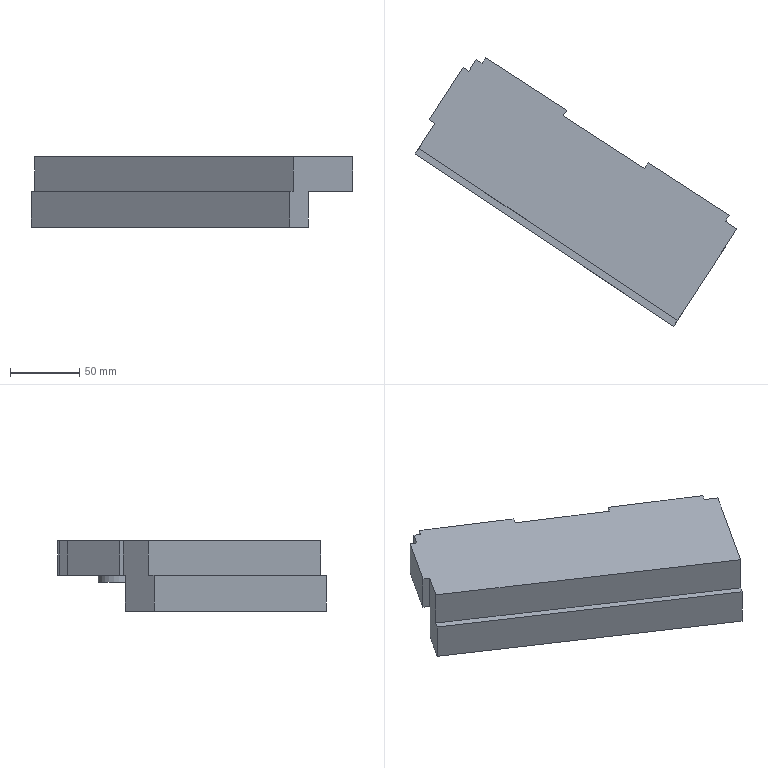Part | NX | features solid 2 | 1 solid | 30 faces | box 233.093 x 194.645 x 51 mm | volume 621496 mm3 | plane 24 | cylinder 4 | spline 2 | commonest cylinder face diameters 30 x4
STEP:
#1=CARTESIAN_POINT('',(545.617,534.28,20.));
#2=VERTEX_POINT('',#1);
#3=CARTESIAN_POINT('',(530.617,534.28,20.));
#4=DIRECTION('',(0.,0.,1.));
#5=DIRECTION('',(1.,0.,0.));
#6=AXIS2_PLACEMENT_3D('',#3,#4,#5);
#7=CIRCLE('',#6,15.);
#8=EDGE_CURVE('',#2,#2,#7,.F.);
#9=ORIENTED_EDGE('',*,*,#8,.F.);
#10=EDGE_LOOP('',(#9));
#11=FACE_BOUND('',#10,.T.);
#12=CARTESIAN_POINT('',(415.617,624.28,20.));
#13=VERTEX_POINT('',#12);
#14=CARTESIAN_POINT('',(400.617,624.28,20.));
#15=DIRECTION('',(0.,0.,1.));
#16=DIRECTION('',(1.,0.,0.));
#17=AXIS2_PLACEMENT_3D('',#14,#15,#16);
#18=CIRCLE('',#17,15.);
#19=EDGE_CURVE('',#13,#13,#18,.F.);
#20=ORIENTED_EDGE('',*,*,#19,.F.);
#21=EDGE_LOOP('',(#20));
#22=FACE_BOUND('',#21,.T.);
#23=CARTESIAN_POINT('',(391.424,667.003,20.));
#24=VERTEX_POINT('',#23);
#25=CARTESIAN_POINT('',(395.617,664.28,20.));
#26=VERTEX_POINT('',#25);
#27=CARTESIAN_POINT('',(-1256.754,1737.343,20.));
#28=DIRECTION('',(0.8387,-0.5446,0.));
#29=VECTOR('',#28,1000.);
#30=LINE('',#27,#29);
#31=EDGE_CURVE('',#24,#26,#30,.T.);
#32=ORIENTED_EDGE('',*,*,#31,.T.);
#33=CARTESIAN_POINT('',(398.341,668.473,20.));
#34=VERTEX_POINT('',#33);
#35=CARTESIAN_POINT('',(395.617,664.28,20.));
#36=DIRECTION('',(0.5446,0.8387,0.));
#37=VECTOR('',#36,1000.);
#38=LINE('',#35,#37);
#39=EDGE_CURVE('',#26,#34,#38,.T.);
#40=ORIENTED_EDGE('',*,*,#39,.T.);
#41=CARTESIAN_POINT('',(457.048,630.348,20.));
#42=VERTEX_POINT('',#41);
#43=CARTESIAN_POINT('',(406.727,663.027,20.));
#44=DIRECTION('',(0.8387,-0.5446,0.));
#45=VECTOR('',#44,1000.);
#46=LINE('',#43,#45);
#47=EDGE_CURVE('',#34,#42,#46,.T.);
#48=ORIENTED_EDGE('',*,*,#47,.T.);
#49=CARTESIAN_POINT('',(454.324,626.155,20.));
#50=VERTEX_POINT('',#49);
#51=CARTESIAN_POINT('',(454.324,626.155,20.));
#52=DIRECTION('',(0.5446,0.8387,0.));
#53=VECTOR('',#52,1000.);
#54=LINE('',#51,#53);
#55=EDGE_CURVE('',#50,#42,#54,.T.);
#56=ORIENTED_EDGE('',*,*,#55,.F.);
#57=CARTESIAN_POINT('',(513.031,588.03,20.));
#58=VERTEX_POINT('',#57);
#59=CARTESIAN_POINT('',(-1256.754,1737.343,20.));
#60=DIRECTION('',(0.8387,-0.5446,0.));
#61=VECTOR('',#60,1000.);
#62=LINE('',#59,#61);
#63=EDGE_CURVE('',#50,#58,#62,.T.);
#64=ORIENTED_EDGE('',*,*,#63,.T.);
#65=CARTESIAN_POINT('',(515.755,592.224,20.));
#66=VERTEX_POINT('',#65);
#67=CARTESIAN_POINT('',(513.031,588.03,20.));
#68=DIRECTION('',(0.5446,0.8387,0.));
#69=VECTOR('',#68,1000.);
#70=LINE('',#67,#69);
#71=EDGE_CURVE('',#58,#66,#70,.T.);
#72=ORIENTED_EDGE('',*,*,#71,.T.);
#73=CARTESIAN_POINT('',(574.461,554.099,20.));
#74=VERTEX_POINT('',#73);
#75=CARTESIAN_POINT('',(545.108,573.161,20.));
#76=DIRECTION('',(0.8387,-0.5446,0.));
#77=VECTOR('',#76,1000.);
#78=LINE('',#75,#77);
#79=EDGE_CURVE('',#66,#74,#78,.T.);
#80=ORIENTED_EDGE('',*,*,#79,.T.);
#81=CARTESIAN_POINT('',(571.738,549.906,20.));
#82=VERTEX_POINT('',#81);
#83=CARTESIAN_POINT('',(571.738,549.906,20.));
#84=DIRECTION('',(0.5446,0.8387,0.));
#85=VECTOR('',#84,1000.);
#86=LINE('',#83,#85);
#87=EDGE_CURVE('',#82,#74,#86,.T.);
#88=ORIENTED_EDGE('',*,*,#87,.F.);
#89=CARTESIAN_POINT('',(580.125,544.459,20.));
#90=VERTEX_POINT('',#89);
#91=CARTESIAN_POINT('',(-1256.754,1737.343,20.));
#92=DIRECTION('',(0.8387,-0.5446,0.));
#93=VECTOR('',#92,1000.);
#94=LINE('',#91,#93);
#95=EDGE_CURVE('',#82,#90,#94,.T.);
#96=ORIENTED_EDGE('',*,*,#95,.T.);
#97=CARTESIAN_POINT('',(547.874,494.797,20.));
#98=VERTEX_POINT('',#97);
#99=CARTESIAN_POINT('',(1248.625,1573.86,20.));
#100=DIRECTION('',(-0.5446,-0.8387,0.));
#101=VECTOR('',#100,1000.);
#102=LINE('',#99,#101);
#103=EDGE_CURVE('',#90,#98,#102,.T.);
#104=ORIENTED_EDGE('',*,*,#103,.T.);
#105=CARTESIAN_POINT('',(360.649,619.614,20.));
#106=VERTEX_POINT('',#105);
#107=CARTESIAN_POINT('',(547.874,494.797,20.));
#108=CARTESIAN_POINT('',(485.466,536.403,20.));
#109=CARTESIAN_POINT('',(423.057,578.008,20.));
#110=CARTESIAN_POINT('',(360.649,619.614,20.));
#111=B_SPLINE_CURVE_WITH_KNOTS('',3,(#107,#108,#109,#110),.UNSPECIFIED.,.F.,.F.,(4,4),(1.354,1.579),.UNSPECIFIED.);
#112=EDGE_CURVE('',#106,#98,#111,.F.);
#113=ORIENTED_EDGE('',*,*,#112,.F.);
#114=CARTESIAN_POINT('',(361.469,620.876,20.));
#115=VERTEX_POINT('',#114);
#116=CARTESIAN_POINT('',(1059.925,1696.404,20.));
#117=DIRECTION('',(-0.5446,-0.8387,0.));
#118=VECTOR('',#117,1000.);
#119=LINE('',#116,#118);
#120=EDGE_CURVE('',#115,#106,#119,.T.);
#121=ORIENTED_EDGE('',*,*,#120,.F.);
#122=CARTESIAN_POINT('',(357.276,623.599,20.));
#123=VERTEX_POINT('',#122);
#124=CARTESIAN_POINT('',(361.469,620.876,20.));
#125=DIRECTION('',(-0.8387,0.5446,0.));
#126=VECTOR('',#125,1000.);
#127=LINE('',#124,#126);
#128=EDGE_CURVE('',#115,#123,#127,.T.);
#129=ORIENTED_EDGE('',*,*,#128,.T.);
#130=CARTESIAN_POINT('',(381.784,661.34,20.));
#131=VERTEX_POINT('',#130);
#132=CARTESIAN_POINT('',(384.508,665.533,20.));
#133=DIRECTION('',(0.5446,0.8387,0.));
#134=VECTOR('',#133,1000.);
#135=LINE('',#132,#134);
#136=EDGE_CURVE('',#123,#131,#135,.T.);
#137=ORIENTED_EDGE('',*,*,#136,.T.);
#138=CARTESIAN_POINT('',(385.978,658.616,20.));
#139=VERTEX_POINT('',#138);
#140=CARTESIAN_POINT('',(385.978,658.616,20.));
#141=DIRECTION('',(-0.8387,0.5446,0.));
#142=VECTOR('',#141,1000.);
#143=LINE('',#140,#142);
#144=EDGE_CURVE('',#139,#131,#143,.T.);
#145=ORIENTED_EDGE('',*,*,#144,.F.);
#146=CARTESIAN_POINT('',(1059.925,1696.404,20.));
#147=DIRECTION('',(-0.5446,-0.8387,0.));
#148=VECTOR('',#147,1000.);
#149=LINE('',#146,#148);
#150=EDGE_CURVE('',#24,#139,#149,.T.);
#151=ORIENTED_EDGE('',*,*,#150,.F.);
#152=EDGE_LOOP('',(#32,#40,#48,#56,#64,#72,#80,#88,#96,#104,#113,#121,#129,#137,#145,#151));
#153=FACE_BOUND('',#152,.T.);
#154=CARTESIAN_POINT('',(515.617,559.28,20.));
#155=VERTEX_POINT('',#154);
#156=CARTESIAN_POINT('',(500.617,559.28,20.));
#157=DIRECTION('',(0.,0.,1.));
#158=DIRECTION('',(1.,0.,0.));
#159=AXIS2_PLACEMENT_3D('',#156,#157,#158);
#160=CIRCLE('',#159,15.);
#161=EDGE_CURVE('',#155,#155,#160,.F.);
#162=ORIENTED_EDGE('',*,*,#161,.F.);
#163=EDGE_LOOP('',(#162));
#164=FACE_BOUND('',#163,.T.);
#165=CARTESIAN_POINT('',(450.617,614.28,20.));
#166=VERTEX_POINT('',#165);
#167=CARTESIAN_POINT('',(435.617,614.28,20.));
#168=DIRECTION('',(0.,0.,1.));
#169=DIRECTION('',(1.,0.,0.));
#170=AXIS2_PLACEMENT_3D('',#167,#168,#169);
#171=CIRCLE('',#170,15.);
#172=EDGE_CURVE('',#166,#166,#171,.F.);
#173=ORIENTED_EDGE('',*,*,#172,.F.);
#174=EDGE_LOOP('',(#173));
#175=FACE_BOUND('',#174,.T.);
#176=CARTESIAN_POINT('',(369.22,631.927,20.));
#177=DIRECTION('',(0.,0.,1.));
#178=DIRECTION('',(1.,0.,0.));
#179=AXIS2_PLACEMENT_3D('',#176,#177,#178);
#180=PLANE('',#179);
#181=ADVANCED_FACE('',(#11,#22,#153,#164,#175),#180,.F.);
#182=ORIENTED_EDGE('',*,*,#95,.F.);
#183=CARTESIAN_POINT('',(571.738,549.906,45.));
#184=VERTEX_POINT('',#183);
#185=CARTESIAN_POINT('',(571.738,549.906,20.));
#186=DIRECTION('',(0.,0.,1.));
#187=VECTOR('',#186,1000.);
#188=LINE('',#185,#187);
#189=EDGE_CURVE('',#82,#184,#188,.T.);
#190=ORIENTED_EDGE('',*,*,#189,.T.);
#191=CARTESIAN_POINT('',(580.125,544.459,45.));
#192=VERTEX_POINT('',#191);
#193=CARTESIAN_POINT('',(-1256.754,1737.343,45.));
#194=DIRECTION('',(0.8387,-0.5446,0.));
#195=VECTOR('',#194,1000.);
#196=LINE('',#193,#195);
#197=EDGE_CURVE('',#184,#192,#196,.T.);
#198=ORIENTED_EDGE('',*,*,#197,.T.);
#199=CARTESIAN_POINT('',(580.125,544.459,70.));
#200=DIRECTION('',(0.,0.,1.));
#201=VECTOR('',#200,1000.);
#202=LINE('',#199,#201);
#203=EDGE_CURVE('',#90,#192,#202,.T.);
#204=ORIENTED_EDGE('',*,*,#203,.F.);
#205=EDGE_LOOP('',(#182,#190,#198,#204));
#206=FACE_BOUND('',#205,.T.);
#207=CARTESIAN_POINT('',(-1256.754,1737.343,70.));
#208=DIRECTION('',(0.5446,0.8387,0.));
#209=DIRECTION('',(-0.8387,0.5446,0.));
#210=AXIS2_PLACEMENT_3D('',#207,#208,#209);
#211=PLANE('',#210);
#212=ADVANCED_FACE('',(#206),#211,.T.);
#213=CARTESIAN_POINT('',(513.031,588.03,45.));
#214=VERTEX_POINT('',#213);
#215=CARTESIAN_POINT('',(513.031,588.03,20.));
#216=DIRECTION('',(0.,0.,-1.));
#217=VECTOR('',#216,1000.);
#218=LINE('',#215,#217);
#219=EDGE_CURVE('',#58,#214,#218,.F.);
#220=ORIENTED_EDGE('',*,*,#219,.F.);
#221=ORIENTED_EDGE('',*,*,#63,.F.);
#222=CARTESIAN_POINT('',(454.324,626.155,45.));
#223=VERTEX_POINT('',#222);
#224=CARTESIAN_POINT('',(454.324,626.155,20.));
#225=DIRECTION('',(0.,0.,1.));
#226=VECTOR('',#225,1000.);
#227=LINE('',#224,#226);
#228=EDGE_CURVE('',#50,#223,#227,.T.);
#229=ORIENTED_EDGE('',*,*,#228,.T.);
#230=CARTESIAN_POINT('',(-1256.754,1737.343,45.));
#231=DIRECTION('',(0.8387,-0.5446,0.));
#232=VECTOR('',#231,1000.);
#233=LINE('',#230,#232);
#234=EDGE_CURVE('',#223,#214,#233,.T.);
#235=ORIENTED_EDGE('',*,*,#234,.T.);
#236=EDGE_LOOP('',(#220,#221,#229,#235));
#237=FACE_BOUND('',#236,.T.);
#238=CARTESIAN_POINT('',(-1256.754,1737.343,70.));
#239=DIRECTION('',(0.5446,0.8387,0.));
#240=DIRECTION('',(-0.8387,0.5446,0.));
#241=AXIS2_PLACEMENT_3D('',#238,#239,#240);
#242=PLANE('',#241);
#243=ADVANCED_FACE('',(#237),#242,.T.);
#244=CARTESIAN_POINT('',(385.978,658.616,45.));
#245=VERTEX_POINT('',#244);
#246=CARTESIAN_POINT('',(385.978,658.616,20.));
#247=DIRECTION('',(0.,0.,1.));
#248=VECTOR('',#247,1000.);
#249=LINE('',#246,#248);
#250=EDGE_CURVE('',#139,#245,#249,.T.);
#251=ORIENTED_EDGE('',*,*,#250,.T.);
#252=CARTESIAN_POINT('',(391.424,667.003,45.));
#253=VERTEX_POINT('',#252);
#254=CARTESIAN_POINT('',(1059.925,1696.404,45.));
#255=DIRECTION('',(-0.5446,-0.8387,0.));
#256=VECTOR('',#255,1000.);
#257=LINE('',#254,#256);
#258=EDGE_CURVE('',#253,#245,#257,.T.);
#259=ORIENTED_EDGE('',*,*,#258,.F.);
#260=CARTESIAN_POINT('',(391.424,667.003,70.));
#261=DIRECTION('',(0.,0.,-1.));
#262=VECTOR('',#261,1000.);
#263=LINE('',#260,#262);
#264=EDGE_CURVE('',#253,#24,#263,.T.);
#265=ORIENTED_EDGE('',*,*,#264,.T.);
#266=ORIENTED_EDGE('',*,*,#150,.T.);
#267=EDGE_LOOP('',(#251,#259,#265,#266));
#268=FACE_BOUND('',#267,.T.);
#269=CARTESIAN_POINT('',(1059.925,1696.404,70.));
#270=DIRECTION('',(0.8387,-0.5446,0.));
#271=DIRECTION('',(0.5446,0.8387,0.));
#272=AXIS2_PLACEMENT_3D('',#269,#270,#271);
#273=PLANE('',#272);
#274=ADVANCED_FACE('',(#268),#273,.F.);
#275=CARTESIAN_POINT('',(395.617,664.28,45.));
#276=VERTEX_POINT('',#275);
#277=CARTESIAN_POINT('',(395.617,664.28,20.));
#278=DIRECTION('',(0.,0.,-1.));
#279=VECTOR('',#278,1000.);
#280=LINE('',#277,#279);
#281=EDGE_CURVE('',#26,#276,#280,.F.);
#282=ORIENTED_EDGE('',*,*,#281,.F.);
#283=ORIENTED_EDGE('',*,*,#31,.F.);
#284=ORIENTED_EDGE('',*,*,#264,.F.);
#285=CARTESIAN_POINT('',(-1256.754,1737.343,45.));
#286=DIRECTION('',(0.8387,-0.5446,0.));
#287=VECTOR('',#286,1000.);
#288=LINE('',#285,#287);
#289=EDGE_CURVE('',#253,#276,#288,.T.);
#290=ORIENTED_EDGE('',*,*,#289,.T.);
#291=EDGE_LOOP('',(#282,#283,#284,#290));
#292=FACE_BOUND('',#291,.T.);
#293=CARTESIAN_POINT('',(-1256.754,1737.343,70.));
#294=DIRECTION('',(0.5446,0.8387,0.));
#295=DIRECTION('',(-0.8387,0.5446,0.));
#296=AXIS2_PLACEMENT_3D('',#293,#294,#295);
#297=PLANE('',#296);
#298=ADVANCED_FACE('',(#292),#297,.T.);
#299=CARTESIAN_POINT('',(361.469,620.876,45.));
#300=VERTEX_POINT('',#299);
#301=CARTESIAN_POINT('',(349.755,602.839,45.));
#302=VERTEX_POINT('',#301);
#303=CARTESIAN_POINT('',(1059.925,1696.404,45.));
#304=DIRECTION('',(-0.5446,-0.8387,0.));
#305=VECTOR('',#304,1000.);
#306=LINE('',#303,#305);
#307=EDGE_CURVE('',#300,#302,#306,.T.);
#308=ORIENTED_EDGE('',*,*,#307,.F.);
#309=CARTESIAN_POINT('',(361.469,620.876,20.));
#310=DIRECTION('',(0.,0.,-1.));
#311=VECTOR('',#310,1000.);
#312=LINE('',#309,#311);
#313=EDGE_CURVE('',#115,#300,#312,.F.);
#314=ORIENTED_EDGE('',*,*,#313,.F.);
#315=ORIENTED_EDGE('',*,*,#120,.T.);
#316=CARTESIAN_POINT('',(360.649,619.614,-6.));
#317=VERTEX_POINT('',#316);
#318=CARTESIAN_POINT('',(360.649,619.614,-6.));
#319=DIRECTION('',(0.,0.,1.));
#320=VECTOR('',#319,1000.);
#321=LINE('',#318,#320);
#322=EDGE_CURVE('',#317,#106,#321,.T.);
#323=ORIENTED_EDGE('',*,*,#322,.F.);
#324=CARTESIAN_POINT('',(347.032,598.645,-6.));
#325=VERTEX_POINT('',#324);
#326=CARTESIAN_POINT('',(1059.925,1696.404,-6.));
#327=DIRECTION('',(-0.5446,-0.8387,0.));
#328=VECTOR('',#327,1000.);
#329=LINE('',#326,#328);
#330=EDGE_CURVE('',#317,#325,#329,.T.);
#331=ORIENTED_EDGE('',*,*,#330,.T.);
#332=CARTESIAN_POINT('',(347.032,598.645,20.));
#333=VERTEX_POINT('',#332);
#334=CARTESIAN_POINT('',(347.032,598.645,70.));
#335=DIRECTION('',(0.,0.,-1.));
#336=VECTOR('',#335,1000.);
#337=LINE('',#334,#336);
#338=EDGE_CURVE('',#333,#325,#337,.T.);
#339=ORIENTED_EDGE('',*,*,#338,.F.);
#340=CARTESIAN_POINT('',(349.755,602.839,20.));
#341=VERTEX_POINT('',#340);
#342=CARTESIAN_POINT('',(347.032,598.645,20.));
#343=DIRECTION('',(0.5446,0.8387,0.));
#344=VECTOR('',#343,1000.);
#345=LINE('',#342,#344);
#346=EDGE_CURVE('',#333,#341,#345,.T.);
#347=ORIENTED_EDGE('',*,*,#346,.T.);
#348=CARTESIAN_POINT('',(349.755,602.839,70.));
#349=DIRECTION('',(0.,0.,1.));
#350=VECTOR('',#349,1000.);
#351=LINE('',#348,#350);
#352=EDGE_CURVE('',#302,#341,#351,.F.);
#353=ORIENTED_EDGE('',*,*,#352,.F.);
#354=EDGE_LOOP('',(#308,#314,#315,#323,#331,#339,#347,#353));
#355=FACE_BOUND('',#354,.T.);
#356=CARTESIAN_POINT('',(1059.925,1696.404,70.));
#357=DIRECTION('',(0.8387,-0.5446,0.));
#358=DIRECTION('',(0.5446,0.8387,0.));
#359=AXIS2_PLACEMENT_3D('',#356,#357,#358);
#360=PLANE('',#359);
#361=ADVANCED_FACE('',(#355),#360,.F.);
#362=ORIENTED_EDGE('',*,*,#103,.F.);
#363=ORIENTED_EDGE('',*,*,#203,.T.);
#364=CARTESIAN_POINT('',(536.98,478.022,45.));
#365=VERTEX_POINT('',#364);
#366=CARTESIAN_POINT('',(1248.625,1573.86,45.));
#367=DIRECTION('',(-0.5446,-0.8387,0.));
#368=VECTOR('',#367,1000.);
#369=LINE('',#366,#368);
#370=EDGE_CURVE('',#192,#365,#369,.T.);
#371=ORIENTED_EDGE('',*,*,#370,.T.);
#372=CARTESIAN_POINT('',(536.98,478.022,20.));
#373=VERTEX_POINT('',#372);
#374=CARTESIAN_POINT('',(536.98,478.022,70.));
#375=DIRECTION('',(0.,0.,1.));
#376=VECTOR('',#375,1000.);
#377=LINE('',#374,#376);
#378=EDGE_CURVE('',#373,#365,#377,.T.);
#379=ORIENTED_EDGE('',*,*,#378,.F.);
#380=CARTESIAN_POINT('',(534.257,473.829,20.));
#381=VERTEX_POINT('',#380);
#382=CARTESIAN_POINT('',(1248.625,1573.86,20.));
#383=DIRECTION('',(-0.5446,-0.8387,0.));
#384=VECTOR('',#383,1000.);
#385=LINE('',#382,#384);
#386=EDGE_CURVE('',#373,#381,#385,.T.);
#387=ORIENTED_EDGE('',*,*,#386,.T.);
#388=CARTESIAN_POINT('',(534.257,473.829,-6.));
#389=VERTEX_POINT('',#388);
#390=CARTESIAN_POINT('',(534.257,473.829,70.));
#391=DIRECTION('',(0.,0.,-1.));
#392=VECTOR('',#391,1000.);
#393=LINE('',#390,#392);
#394=EDGE_CURVE('',#381,#389,#393,.T.);
#395=ORIENTED_EDGE('',*,*,#394,.T.);
#396=CARTESIAN_POINT('',(547.874,494.797,-6.));
#397=VERTEX_POINT('',#396);
#398=CARTESIAN_POINT('',(1248.625,1573.86,-6.));
#399=DIRECTION('',(-0.5446,-0.8387,0.));
#400=VECTOR('',#399,1000.);
#401=LINE('',#398,#400);
#402=EDGE_CURVE('',#397,#389,#401,.T.);
#403=ORIENTED_EDGE('',*,*,#402,.F.);
#404=CARTESIAN_POINT('',(547.874,494.797,19.5));
#405=DIRECTION('',(0.,0.,1.));
#406=VECTOR('',#405,1000.);
#407=LINE('',#404,#406);
#408=EDGE_CURVE('',#98,#397,#407,.F.);
#409=ORIENTED_EDGE('',*,*,#408,.F.);
#410=EDGE_LOOP('',(#362,#363,#371,#379,#387,#395,#403,#409));
#411=FACE_BOUND('',#410,.T.);
#412=CARTESIAN_POINT('',(1248.625,1573.86,70.));
#413=DIRECTION('',(0.8387,-0.5446,0.));
#414=DIRECTION('',(0.5446,0.8387,0.));
#415=AXIS2_PLACEMENT_3D('',#412,#413,#414);
#416=PLANE('',#415);
#417=ADVANCED_FACE('',(#411),#416,.T.);
#418=ORIENTED_EDGE('',*,*,#330,.F.);
#419=CARTESIAN_POINT('',(360.649,619.614,-6.));
#420=CARTESIAN_POINT('',(423.057,578.008,-6.));
#421=CARTESIAN_POINT('',(485.466,536.403,-6.));
#422=CARTESIAN_POINT('',(547.874,494.797,-6.));
#423=B_SPLINE_CURVE_WITH_KNOTS('',3,(#419,#420,#421,#422),.UNSPECIFIED.,.F.,.F.,(4,4),(0.,0.225),.UNSPECIFIED.);
#424=EDGE_CURVE('',#317,#397,#423,.T.);
#425=ORIENTED_EDGE('',*,*,#424,.T.);
#426=ORIENTED_EDGE('',*,*,#402,.T.);
#427=CARTESIAN_POINT('',(347.032,598.645,-6.));
#428=DIRECTION('',(0.8321,-0.5547,0.));
#429=VECTOR('',#428,1000.);
#430=LINE('',#427,#429);
#431=EDGE_CURVE('',#325,#389,#430,.T.);
#432=ORIENTED_EDGE('',*,*,#431,.F.);
#433=EDGE_LOOP('',(#418,#425,#426,#432));
#434=FACE_BOUND('',#433,.T.);
#435=CARTESIAN_POINT('',(354.645,1410.288,-6.));
#436=DIRECTION('',(0.,0.,1.));
#437=DIRECTION('',(1.,0.,0.));
#438=AXIS2_PLACEMENT_3D('',#435,#436,#437);
#439=PLANE('',#438);
#440=ADVANCED_FACE('',(#434),#439,.F.);
#441=CARTESIAN_POINT('',(347.032,598.645,20.));
#442=DIRECTION('',(0.8321,-0.5547,0.));
#443=VECTOR('',#442,1000.);
#444=LINE('',#441,#443);
#445=EDGE_CURVE('',#333,#381,#444,.T.);
#446=ORIENTED_EDGE('',*,*,#445,.F.);
#447=ORIENTED_EDGE('',*,*,#338,.T.);
#448=ORIENTED_EDGE('',*,*,#431,.T.);
#449=ORIENTED_EDGE('',*,*,#394,.F.);
#450=EDGE_LOOP('',(#446,#447,#448,#449));
#451=FACE_BOUND('',#450,.T.);
#452=CARTESIAN_POINT('',(347.032,598.645,70.));
#453=DIRECTION('',(0.5547,0.8321,0.));
#454=DIRECTION('',(-0.8321,0.5547,0.));
#455=AXIS2_PLACEMENT_3D('',#452,#453,#454);
#456=PLANE('',#455);
#457=ADVANCED_FACE('',(#451),#456,.F.);
#458=ORIENTED_EDGE('',*,*,#370,.F.);
#459=ORIENTED_EDGE('',*,*,#197,.F.);
#460=CARTESIAN_POINT('',(574.461,554.099,45.));
#461=VERTEX_POINT('',#460);
#462=CARTESIAN_POINT('',(571.738,549.906,45.));
#463=DIRECTION('',(0.5446,0.8387,0.));
#464=VECTOR('',#463,1000.);
#465=LINE('',#462,#464);
#466=EDGE_CURVE('',#184,#461,#465,.T.);
#467=ORIENTED_EDGE('',*,*,#466,.T.);
#468=CARTESIAN_POINT('',(515.755,592.224,45.));
#469=VERTEX_POINT('',#468);
#470=CARTESIAN_POINT('',(545.108,573.161,45.));
#471=DIRECTION('',(0.8387,-0.5446,0.));
#472=VECTOR('',#471,1000.);
#473=LINE('',#470,#472);
#474=EDGE_CURVE('',#469,#461,#473,.T.);
#475=ORIENTED_EDGE('',*,*,#474,.F.);
#476=CARTESIAN_POINT('',(513.031,588.03,45.));
#477=DIRECTION('',(0.5446,0.8387,0.));
#478=VECTOR('',#477,1000.);
#479=LINE('',#476,#478);
#480=EDGE_CURVE('',#214,#469,#479,.T.);
#481=ORIENTED_EDGE('',*,*,#480,.F.);
#482=ORIENTED_EDGE('',*,*,#234,.F.);
#483=CARTESIAN_POINT('',(457.048,630.348,45.));
#484=VERTEX_POINT('',#483);
#485=CARTESIAN_POINT('',(454.324,626.155,45.));
#486=DIRECTION('',(0.5446,0.8387,0.));
#487=VECTOR('',#486,1000.);
#488=LINE('',#485,#487);
#489=EDGE_CURVE('',#223,#484,#488,.T.);
#490=ORIENTED_EDGE('',*,*,#489,.T.);
#491=CARTESIAN_POINT('',(398.341,668.473,45.));
#492=VERTEX_POINT('',#491);
#493=CARTESIAN_POINT('',(406.727,663.027,45.));
#494=DIRECTION('',(0.8387,-0.5446,0.));
#495=VECTOR('',#494,1000.);
#496=LINE('',#493,#495);
#497=EDGE_CURVE('',#492,#484,#496,.T.);
#498=ORIENTED_EDGE('',*,*,#497,.F.);
#499=CARTESIAN_POINT('',(395.617,664.28,45.));
#500=DIRECTION('',(0.5446,0.8387,0.));
#501=VECTOR('',#500,1000.);
#502=LINE('',#499,#501);
#503=EDGE_CURVE('',#276,#492,#502,.T.);
#504=ORIENTED_EDGE('',*,*,#503,.F.);
#505=ORIENTED_EDGE('',*,*,#289,.F.);
#506=ORIENTED_EDGE('',*,*,#258,.T.);
#507=CARTESIAN_POINT('',(381.784,661.34,45.));
#508=VERTEX_POINT('',#507);
#509=CARTESIAN_POINT('',(385.978,658.616,45.));
#510=DIRECTION('',(-0.8387,0.5446,0.));
#511=VECTOR('',#510,1000.);
#512=LINE('',#509,#511);
#513=EDGE_CURVE('',#245,#508,#512,.T.);
#514=ORIENTED_EDGE('',*,*,#513,.T.);
#515=CARTESIAN_POINT('',(357.276,623.599,45.));
#516=VERTEX_POINT('',#515);
#517=CARTESIAN_POINT('',(384.508,665.533,45.));
#518=DIRECTION('',(-0.5446,-0.8387,0.));
#519=VECTOR('',#518,1000.);
#520=LINE('',#517,#519);
#521=EDGE_CURVE('',#516,#508,#520,.F.);
#522=ORIENTED_EDGE('',*,*,#521,.F.);
#523=CARTESIAN_POINT('',(361.469,620.876,45.));
#524=DIRECTION('',(-0.8387,0.5446,0.));
#525=VECTOR('',#524,1000.);
#526=LINE('',#523,#525);
#527=EDGE_CURVE('',#300,#516,#526,.T.);
#528=ORIENTED_EDGE('',*,*,#527,.F.);
#529=ORIENTED_EDGE('',*,*,#307,.T.);
#530=CARTESIAN_POINT('',(349.755,602.839,45.));
#531=CARTESIAN_POINT('',(412.164,561.233,45.));
#532=CARTESIAN_POINT('',(474.572,519.628,45.));
#533=CARTESIAN_POINT('',(536.98,478.022,45.));
#534=B_SPLINE_CURVE_WITH_KNOTS('',3,(#530,#531,#532,#533),.UNSPECIFIED.,.F.,.F.,(4,4),(0.,1.),.UNSPECIFIED.);
#535=EDGE_CURVE('',#302,#365,#534,.T.);
#536=ORIENTED_EDGE('',*,*,#535,.T.);
#537=EDGE_LOOP('',(#458,#459,#467,#475,#481,#482,#490,#498,#504,#505,#506,#514,#522,#528,#529,#536));
#538=FACE_BOUND('',#537,.T.);
#539=CARTESIAN_POINT('',(354.645,1410.288,45.));
#540=DIRECTION('',(0.,0.,1.));
#541=DIRECTION('',(1.,0.,0.));
#542=AXIS2_PLACEMENT_3D('',#539,#540,#541);
#543=PLANE('',#542);
#544=ADVANCED_FACE('',(#538),#543,.T.);
#545=ORIENTED_EDGE('',*,*,#378,.T.);
#546=ORIENTED_EDGE('',*,*,#535,.F.);
#547=ORIENTED_EDGE('',*,*,#352,.T.);
#548=CARTESIAN_POINT('',(349.755,602.839,20.));
#549=CARTESIAN_POINT('',(412.164,561.233,20.));
#550=CARTESIAN_POINT('',(474.572,519.628,20.));
#551=CARTESIAN_POINT('',(536.98,478.022,20.));
#552=B_SPLINE_CURVE_WITH_KNOTS('',3,(#548,#549,#550,#551),.UNSPECIFIED.,.F.,.F.,(4,4),(0.3568,0.5818),.UNSPECIFIED.);
#553=EDGE_CURVE('',#341,#373,#552,.T.);
#554=ORIENTED_EDGE('',*,*,#553,.T.);
#555=EDGE_LOOP('',(#545,#546,#547,#554));
#556=FACE_BOUND('',#555,.T.);
#557=CARTESIAN_POINT('',(349.755,602.839,20.));
#558=CARTESIAN_POINT('',(349.755,602.839,45.));
#559=CARTESIAN_POINT('',(416.535,558.32,20.));
#560=CARTESIAN_POINT('',(416.535,558.32,45.));
#561=CARTESIAN_POINT('',(470.669,522.23,20.));
#562=CARTESIAN_POINT('',(470.669,522.23,45.));
#563=CARTESIAN_POINT('',(536.98,478.022,20.));
#564=CARTESIAN_POINT('',(536.98,478.022,45.));
#565=B_SPLINE_SURFACE_WITH_KNOTS('',3,1,((#557,#558),(#559,#560),(#561,#562),(#563,#564)),.SURF_OF_LINEAR_EXTRUSION.,.F.,.F.,.F.,(4,4),(2,2),(-0.0002501,0.9997),(0.,1.),.PIECEWISE_BEZIER_KNOTS.);
#566=ADVANCED_FACE('',(#556),#565,.T.);
#567=ORIENTED_EDGE('',*,*,#553,.F.);
#568=ORIENTED_EDGE('',*,*,#346,.F.);
#569=ORIENTED_EDGE('',*,*,#445,.T.);
#570=ORIENTED_EDGE('',*,*,#386,.F.);
#571=EDGE_LOOP('',(#567,#568,#569,#570));
#572=FACE_BOUND('',#571,.T.);
#573=CARTESIAN_POINT('',(347.032,598.645,20.));
#574=DIRECTION('',(0.,0.,1.));
#575=DIRECTION('',(1.,0.,0.));
#576=AXIS2_PLACEMENT_3D('',#573,#574,#575);
#577=PLANE('',#576);
#578=ADVANCED_FACE('',(#572),#577,.T.);
#579=ORIENTED_EDGE('',*,*,#424,.F.);
#580=ORIENTED_EDGE('',*,*,#322,.T.);
#581=ORIENTED_EDGE('',*,*,#112,.T.);
#582=ORIENTED_EDGE('',*,*,#408,.T.);
#583=EDGE_LOOP('',(#579,#580,#581,#582));
#584=FACE_BOUND('',#583,.T.);
#585=CARTESIAN_POINT('',(360.649,619.614,-6.));
#586=CARTESIAN_POINT('',(360.649,619.614,20.));
#587=CARTESIAN_POINT('',(427.428,575.095,-6.));
#588=CARTESIAN_POINT('',(427.428,575.095,20.));
#589=CARTESIAN_POINT('',(481.588,538.988,-6.));
#590=CARTESIAN_POINT('',(481.588,538.988,20.));
#591=CARTESIAN_POINT('',(547.874,494.797,-6.));
#592=CARTESIAN_POINT('',(547.874,494.797,20.));
#593=B_SPLINE_SURFACE_WITH_KNOTS('',3,1,((#585,#586),(#587,#588),(#589,#590),(#591,#592)),.SURF_OF_LINEAR_EXTRUSION.,.F.,.F.,.F.,(4,4),(2,2),(-0.001251,0.9987),(0.,1.),.PIECEWISE_BEZIER_KNOTS.);
#594=ADVANCED_FACE('',(#584),#593,.F.);
#595=CARTESIAN_POINT('',(381.784,661.34,20.));
#596=DIRECTION('',(0.,0.,1.));
#597=VECTOR('',#596,1000.);
#598=LINE('',#595,#597);
#599=EDGE_CURVE('',#131,#508,#598,.T.);
#600=ORIENTED_EDGE('',*,*,#599,.T.);
#601=ORIENTED_EDGE('',*,*,#513,.F.);
#602=ORIENTED_EDGE('',*,*,#250,.F.);
#603=ORIENTED_EDGE('',*,*,#144,.T.);
#604=EDGE_LOOP('',(#600,#601,#602,#603));
#605=FACE_BOUND('',#604,.T.);
#606=CARTESIAN_POINT('',(385.978,658.616,20.));
#607=DIRECTION('',(-0.5446,-0.8387,0.));
#608=DIRECTION('',(0.8387,-0.5446,0.));
#609=AXIS2_PLACEMENT_3D('',#606,#607,#608);
#610=PLANE('',#609);
#611=ADVANCED_FACE('',(#605),#610,.F.);
#612=CARTESIAN_POINT('',(357.276,623.599,20.));
#613=DIRECTION('',(0.,0.,-1.));
#614=VECTOR('',#613,1000.);
#615=LINE('',#612,#614);
#616=EDGE_CURVE('',#123,#516,#615,.F.);
#617=ORIENTED_EDGE('',*,*,#616,.F.);
#618=ORIENTED_EDGE('',*,*,#128,.F.);
#619=ORIENTED_EDGE('',*,*,#313,.T.);
#620=ORIENTED_EDGE('',*,*,#527,.T.);
#621=EDGE_LOOP('',(#617,#618,#619,#620));
#622=FACE_BOUND('',#621,.T.);
#623=CARTESIAN_POINT('',(361.469,620.876,20.));
#624=DIRECTION('',(-0.5446,-0.8387,0.));
#625=DIRECTION('',(0.8387,-0.5446,0.));
#626=AXIS2_PLACEMENT_3D('',#623,#624,#625);
#627=PLANE('',#626);
#628=ADVANCED_FACE('',(#622),#627,.T.);
#629=ORIENTED_EDGE('',*,*,#599,.F.);
#630=ORIENTED_EDGE('',*,*,#136,.F.);
#631=ORIENTED_EDGE('',*,*,#616,.T.);
#632=ORIENTED_EDGE('',*,*,#521,.T.);
#633=EDGE_LOOP('',(#629,#630,#631,#632));
#634=FACE_BOUND('',#633,.T.);
#635=CARTESIAN_POINT('',(384.508,665.533,20.));
#636=DIRECTION('',(-0.8387,0.5446,0.));
#637=DIRECTION('',(0.,0.,1.));
#638=AXIS2_PLACEMENT_3D('',#635,#636,#637);
#639=PLANE('',#638);
#640=ADVANCED_FACE('',(#634),#639,.T.);
#641=CARTESIAN_POINT('',(457.048,630.348,20.));
#642=DIRECTION('',(0.,0.,1.));
#643=VECTOR('',#642,1000.);
#644=LINE('',#641,#643);
#645=EDGE_CURVE('',#42,#484,#644,.T.);
#646=ORIENTED_EDGE('',*,*,#645,.T.);
#647=ORIENTED_EDGE('',*,*,#489,.F.);
#648=ORIENTED_EDGE('',*,*,#228,.F.);
#649=ORIENTED_EDGE('',*,*,#55,.T.);
#650=EDGE_LOOP('',(#646,#647,#648,#649));
#651=FACE_BOUND('',#650,.T.);
#652=CARTESIAN_POINT('',(454.324,626.155,20.));
#653=DIRECTION('',(-0.8387,0.5446,0.));
#654=DIRECTION('',(-0.5446,-0.8387,0.));
#655=AXIS2_PLACEMENT_3D('',#652,#653,#654);
#656=PLANE('',#655);
#657=ADVANCED_FACE('',(#651),#656,.F.);
#658=CARTESIAN_POINT('',(398.341,668.473,20.));
#659=DIRECTION('',(0.,0.,-1.));
#660=VECTOR('',#659,1000.);
#661=LINE('',#658,#660);
#662=EDGE_CURVE('',#34,#492,#661,.F.);
#663=ORIENTED_EDGE('',*,*,#662,.F.);
#664=ORIENTED_EDGE('',*,*,#39,.F.);
#665=ORIENTED_EDGE('',*,*,#281,.T.);
#666=ORIENTED_EDGE('',*,*,#503,.T.);
#667=EDGE_LOOP('',(#663,#664,#665,#666));
#668=FACE_BOUND('',#667,.T.);
#669=CARTESIAN_POINT('',(395.617,664.28,20.));
#670=DIRECTION('',(-0.8387,0.5446,0.));
#671=DIRECTION('',(-0.5446,-0.8387,0.));
#672=AXIS2_PLACEMENT_3D('',#669,#670,#671);
#673=PLANE('',#672);
#674=ADVANCED_FACE('',(#668),#673,.T.);
#675=ORIENTED_EDGE('',*,*,#645,.F.);
#676=ORIENTED_EDGE('',*,*,#47,.F.);
#677=ORIENTED_EDGE('',*,*,#662,.T.);
#678=ORIENTED_EDGE('',*,*,#497,.T.);
#679=EDGE_LOOP('',(#675,#676,#677,#678));
#680=FACE_BOUND('',#679,.T.);
#681=CARTESIAN_POINT('',(406.727,663.027,20.));
#682=DIRECTION('',(0.5446,0.8387,0.));
#683=DIRECTION('',(0.,0.,1.));
#684=AXIS2_PLACEMENT_3D('',#681,#682,#683);
#685=PLANE('',#684);
#686=ADVANCED_FACE('',(#680),#685,.T.);
#687=CARTESIAN_POINT('',(574.461,554.099,20.));
#688=DIRECTION('',(0.,0.,1.));
#689=VECTOR('',#688,1000.);
#690=LINE('',#687,#689);
#691=EDGE_CURVE('',#74,#461,#690,.T.);
#692=ORIENTED_EDGE('',*,*,#691,.T.);
#693=ORIENTED_EDGE('',*,*,#466,.F.);
#694=ORIENTED_EDGE('',*,*,#189,.F.);
#695=ORIENTED_EDGE('',*,*,#87,.T.);
#696=EDGE_LOOP('',(#692,#693,#694,#695));
#697=FACE_BOUND('',#696,.T.);
#698=CARTESIAN_POINT('',(571.738,549.906,20.));
#699=DIRECTION('',(-0.8387,0.5446,0.));
#700=DIRECTION('',(-0.5446,-0.8387,0.));
#701=AXIS2_PLACEMENT_3D('',#698,#699,#700);
#702=PLANE('',#701);
#703=ADVANCED_FACE('',(#697),#702,.F.);
#704=CARTESIAN_POINT('',(515.755,592.224,20.));
#705=DIRECTION('',(0.,0.,-1.));
#706=VECTOR('',#705,1000.);
#707=LINE('',#704,#706);
#708=EDGE_CURVE('',#66,#469,#707,.F.);
#709=ORIENTED_EDGE('',*,*,#708,.F.);
#710=ORIENTED_EDGE('',*,*,#71,.F.);
#711=ORIENTED_EDGE('',*,*,#219,.T.);
#712=ORIENTED_EDGE('',*,*,#480,.T.);
#713=EDGE_LOOP('',(#709,#710,#711,#712));
#714=FACE_BOUND('',#713,.T.);
#715=CARTESIAN_POINT('',(513.031,588.03,20.));
#716=DIRECTION('',(-0.8387,0.5446,0.));
#717=DIRECTION('',(-0.5446,-0.8387,0.));
#718=AXIS2_PLACEMENT_3D('',#715,#716,#717);
#719=PLANE('',#718);
#720=ADVANCED_FACE('',(#714),#719,.T.);
#721=ORIENTED_EDGE('',*,*,#691,.F.);
#722=ORIENTED_EDGE('',*,*,#79,.F.);
#723=ORIENTED_EDGE('',*,*,#708,.T.);
#724=ORIENTED_EDGE('',*,*,#474,.T.);
#725=EDGE_LOOP('',(#721,#722,#723,#724));
#726=FACE_BOUND('',#725,.T.);
#727=CARTESIAN_POINT('',(545.108,573.161,20.));
#728=DIRECTION('',(0.5446,0.8387,0.));
#729=DIRECTION('',(0.,0.,1.));
#730=AXIS2_PLACEMENT_3D('',#727,#728,#729);
#731=PLANE('',#730);
#732=ADVANCED_FACE('',(#726),#731,.T.);
#733=CARTESIAN_POINT('',(415.617,624.28,15.));
#734=VERTEX_POINT('',#733);
#735=CARTESIAN_POINT('',(400.617,624.28,15.));
#736=DIRECTION('',(0.,0.,-1.));
#737=DIRECTION('',(1.,0.,0.));
#738=AXIS2_PLACEMENT_3D('',#735,#736,#737);
#739=CIRCLE('',#738,15.);
#740=EDGE_CURVE('',#734,#734,#739,.T.);
#741=ORIENTED_EDGE('',*,*,#740,.F.);
#742=EDGE_LOOP('',(#741));
#743=FACE_BOUND('',#742,.T.);
#744=ORIENTED_EDGE('',*,*,#19,.T.);
#745=EDGE_LOOP('',(#744));
#746=FACE_BOUND('',#745,.T.);
#747=CARTESIAN_POINT('',(400.617,624.28,15.));
#748=DIRECTION('',(0.,0.,1.));
#749=DIRECTION('',(1.,0.,0.));
#750=AXIS2_PLACEMENT_3D('',#747,#748,#749);
#751=CYLINDRICAL_SURFACE('',#750,15.);
#752=ADVANCED_FACE('',(#743,#746),#751,.T.);
#753=ORIENTED_EDGE('',*,*,#740,.T.);
#754=EDGE_LOOP('',(#753));
#755=FACE_BOUND('',#754,.T.);
#756=CARTESIAN_POINT('',(400.617,624.28,15.));
#757=DIRECTION('',(0.,0.,-1.));
#758=DIRECTION('',(-1.,0.,0.));
#759=AXIS2_PLACEMENT_3D('',#756,#757,#758);
#760=PLANE('',#759);
#761=ADVANCED_FACE('',(#755),#760,.T.);
#762=CARTESIAN_POINT('',(515.617,559.28,15.));
#763=VERTEX_POINT('',#762);
#764=CARTESIAN_POINT('',(500.617,559.28,15.));
#765=DIRECTION('',(0.,0.,-1.));
#766=DIRECTION('',(1.,0.,0.));
#767=AXIS2_PLACEMENT_3D('',#764,#765,#766);
#768=CIRCLE('',#767,15.);
#769=EDGE_CURVE('',#763,#763,#768,.T.);
#770=ORIENTED_EDGE('',*,*,#769,.F.);
#771=EDGE_LOOP('',(#770));
#772=FACE_BOUND('',#771,.T.);
#773=ORIENTED_EDGE('',*,*,#161,.T.);
#774=EDGE_LOOP('',(#773));
#775=FACE_BOUND('',#774,.T.);
#776=CARTESIAN_POINT('',(500.617,559.28,15.));
#777=DIRECTION('',(0.,0.,1.));
#778=DIRECTION('',(1.,0.,0.));
#779=AXIS2_PLACEMENT_3D('',#776,#777,#778);
#780=CYLINDRICAL_SURFACE('',#779,15.);
#781=ADVANCED_FACE('',(#772,#775),#780,.T.);
#782=ORIENTED_EDGE('',*,*,#769,.T.);
#783=EDGE_LOOP('',(#782));
#784=FACE_BOUND('',#783,.T.);
#785=CARTESIAN_POINT('',(500.617,559.28,15.));
#786=DIRECTION('',(0.,0.,-1.));
#787=DIRECTION('',(-1.,0.,0.));
#788=AXIS2_PLACEMENT_3D('',#785,#786,#787);
#789=PLANE('',#788);
#790=ADVANCED_FACE('',(#784),#789,.T.);
#791=CARTESIAN_POINT('',(545.617,534.28,15.));
#792=VERTEX_POINT('',#791);
#793=CARTESIAN_POINT('',(530.617,534.28,15.));
#794=DIRECTION('',(0.,0.,-1.));
#795=DIRECTION('',(1.,0.,0.));
#796=AXIS2_PLACEMENT_3D('',#793,#794,#795);
#797=CIRCLE('',#796,15.);
#798=EDGE_CURVE('',#792,#792,#797,.T.);
#799=ORIENTED_EDGE('',*,*,#798,.F.);
#800=EDGE_LOOP('',(#799));
#801=FACE_BOUND('',#800,.T.);
#802=ORIENTED_EDGE('',*,*,#8,.T.);
#803=EDGE_LOOP('',(#802));
#804=FACE_BOUND('',#803,.T.);
#805=CARTESIAN_POINT('',(530.617,534.28,15.));
#806=DIRECTION('',(0.,0.,1.));
#807=DIRECTION('',(1.,0.,0.));
#808=AXIS2_PLACEMENT_3D('',#805,#806,#807);
#809=CYLINDRICAL_SURFACE('',#808,15.);
#810=ADVANCED_FACE('',(#801,#804),#809,.T.);
#811=ORIENTED_EDGE('',*,*,#798,.T.);
#812=EDGE_LOOP('',(#811));
#813=FACE_BOUND('',#812,.T.);
#814=CARTESIAN_POINT('',(530.617,534.28,15.));
#815=DIRECTION('',(0.,0.,-1.));
#816=DIRECTION('',(-1.,0.,0.));
#817=AXIS2_PLACEMENT_3D('',#814,#815,#816);
#818=PLANE('',#817);
#819=ADVANCED_FACE('',(#813),#818,.T.);
#820=CARTESIAN_POINT('',(450.617,614.28,15.));
#821=VERTEX_POINT('',#820);
#822=CARTESIAN_POINT('',(435.617,614.28,15.));
#823=DIRECTION('',(0.,0.,-1.));
#824=DIRECTION('',(1.,0.,0.));
#825=AXIS2_PLACEMENT_3D('',#822,#823,#824);
#826=CIRCLE('',#825,15.);
#827=EDGE_CURVE('',#821,#821,#826,.T.);
#828=ORIENTED_EDGE('',*,*,#827,.F.);
#829=EDGE_LOOP('',(#828));
#830=FACE_BOUND('',#829,.T.);
#831=ORIENTED_EDGE('',*,*,#172,.T.);
#832=EDGE_LOOP('',(#831));
#833=FACE_BOUND('',#832,.T.);
#834=CARTESIAN_POINT('',(435.617,614.28,15.));
#835=DIRECTION('',(0.,0.,1.));
#836=DIRECTION('',(1.,0.,0.));
#837=AXIS2_PLACEMENT_3D('',#834,#835,#836);
#838=CYLINDRICAL_SURFACE('',#837,15.);
#839=ADVANCED_FACE('',(#830,#833),#838,.T.);
#840=ORIENTED_EDGE('',*,*,#827,.T.);
#841=EDGE_LOOP('',(#840));
#842=FACE_BOUND('',#841,.T.);
#843=CARTESIAN_POINT('',(435.617,614.28,15.));
#844=DIRECTION('',(0.,0.,-1.));
#845=DIRECTION('',(-1.,0.,0.));
#846=AXIS2_PLACEMENT_3D('',#843,#844,#845);
#847=PLANE('',#846);
#848=ADVANCED_FACE('',(#842),#847,.T.);
#849=CLOSED_SHELL('',(#181,#212,#243,#274,#298,#361,#417,#440,#457,#544,#566,#578,#594,#611,#628,#640,#657,#674,#686,#703,#720,#732,#752,#761,#781,#790,#810,#819,#839,#848));
#850=MANIFOLD_SOLID_BREP('',#849);
#851=(LENGTH_UNIT()NAMED_UNIT(*)SI_UNIT(.MILLI.,.METRE.));
#852=UNCERTAINTY_MEASURE_WITH_UNIT(LENGTH_MEASURE(0.0508),#851,'','');
#853=(NAMED_UNIT(*)PLANE_ANGLE_UNIT()SI_UNIT($,.RADIAN.));
#854=(NAMED_UNIT(*)SI_UNIT($,.STERADIAN.)SOLID_ANGLE_UNIT());
#855=(GEOMETRIC_REPRESENTATION_CONTEXT(3)GLOBAL_UNCERTAINTY_ASSIGNED_CONTEXT((#852))GLOBAL_UNIT_ASSIGNED_CONTEXT((#851,#853,#854))REPRESENTATION_CONTEXT('',''));
#856=ADVANCED_BREP_SHAPE_REPRESENTATION('',(#850),#855);